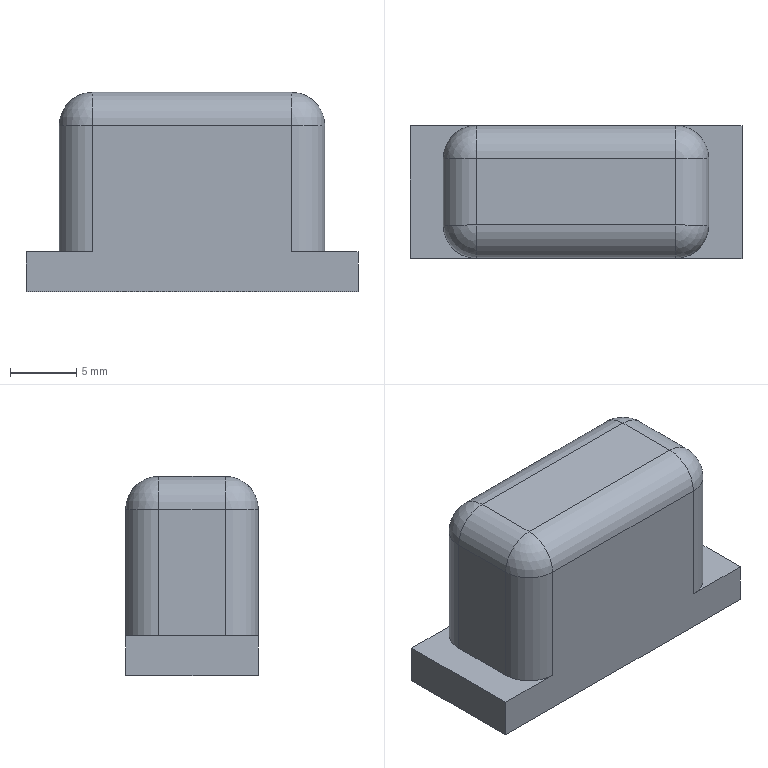NC program | NX | posted with a generic post | part box 25 x 10 x 15 mm
Lines 1366 to 3091 of 3091, first 1419 of 1722 lines:
(ZLEVEL_PROFILE_COPY_1 , TOOL : D4R0.5)
N2712 T05 M6
N2714 G54
N2716 G17 G0 G90 X1.318 Y-4.221 S7500 M3
N2718 G43 Z30. H5
N2720 Z1.
N2722 G94 G1 X-7.5 Z0.538 F1000.
N2724 X-7.686 Z0.528
N2726 X-8.139 Y-4.108 Z0.504
N2728 X-8.546 Y-3.879 Z0.479
N2730 X-8.877 Y-3.548 Z0.455
N2732 X-9.108 Y-3.142 Z0.43
N2734 X-9.221 Y-2.688 Z0.406
N2736 Y-2.502 Z0.396
N2738 Y2.502 Z0.134
N2740 Y2.688 Z0.124
N2742 X-9.108 Y3.141 Z0.099
N2744 X-8.878 Y3.547 Z0.075
N2746 X-8.548 Y3.877 Z0.051
N2748 X-8.142 Y4.107 Z0.026
N2750 X-7.689 Y4.221 Z0.002
N2752 X-7.503 Z-0.008
N2754 X7.503 F3000.
N2756 G2 X9.221 Y2.5 R1.721
N2758 G1 Y-2.5
N2760 G2 X7.5 Y-4.221 R1.721
N2762 G1 X-7.5
N2764 G2 X-9.221 Y-2.502 R1.721
N2766 G1 Y2.502
N2768 G2 X-7.503 Y4.221 R1.721
N2770 G1 X-7.401 Y4.244 Z-0.01
N2772 X-7.298 Y4.265 Z-0.012
N2774 X-7.195 Y4.285 Z-0.014
N2776 X-7.093 Y4.303 Z-0.015
N2778 X-6.99 Y4.32 Z-0.017
N2780 X-6.887 Y4.336 Z-0.019
N2782 X7.492
N2784 G2 X9.336 Y2.5 R1.836
N2786 G1 Y-2.5
N2788 G2 X7.5 Y-4.336 R1.836
N2790 G1 X-7.5
N2792 G2 X-9.336 Y-2.502 R1.836
N2794 G1 Y2.502
N2796 G2 X-7.504 Y4.336 R1.836
N2798 G1 X-7.367 Y4.357 Z-0.021
N2800 X-7.231 Y4.376 Z-0.024
N2802 X-7.094 Y4.394 Z-0.026
N2804 X-6.958 Y4.412 Z-0.028
N2806 X-6.821 Y4.429 Z-0.031
N2808 X-6.685 Y4.445 Z-0.033
N2810 X7.497
N2812 G2 X9.445 Y2.5 R1.945
N2814 G1 Y-2.5
N2816 G2 X7.5 Y-4.445 R1.945
N2818 G1 X-7.5
N2820 G2 X-9.445 Y-2.502 R1.945
N2822 G1 Y2.502
N2824 G2 X-7.504 Y4.445 R1.945
N2826 G1 X-7.379 Y4.459 Z-0.035
N2828 X-7.254 Y4.473 Z-0.038
N2830 X-7.129 Y4.487 Z-0.04
N2832 X-7.004 Y4.5 Z-0.042
N2834 X-6.88 Y4.512 Z-0.044
N2836 X-6.755 Y4.525 Z-0.046
N2838 X-6.63 Y4.537 Z-0.048
N2840 X-6.505 Y4.549 Z-0.051
N2842 X7.493
N2844 G2 X9.549 Y2.5 R2.049
N2846 G1 Y-2.5
N2848 G2 X7.5 Y-4.549 R2.049
N2850 G1 X-7.5
N2852 G2 X-9.549 Y-2.502 R2.049
N2854 G1 Y2.502
N2856 G2 X-7.504 Y4.549 R2.049
N2858 G1 X-7.385 Y4.56 Z-0.053
N2860 X-7.266 Y4.571 Z-0.055
N2862 X-7.146 Y4.581 Z-0.057
N2864 X-7.027 Y4.592 Z-0.059
N2866 X-6.908 Y4.602 Z-0.061
N2868 X-6.788 Y4.612 Z-0.063
N2870 X-6.669 Y4.622 Z-0.065
N2872 X-6.55 Y4.632 Z-0.067
N2874 X-6.431 Y4.641 Z-0.069
N2876 X-6.311 Y4.651 Z-0.071
N2878 X7.497
N2880 G2 X9.651 Y2.5 R2.151
N2882 G1 Y-2.5
N2884 G2 X7.5 Y-4.651 R2.151
N2886 G1 X-7.5
N2888 G2 X-9.651 Y-2.502 R2.151
N2890 G1 Y2.502
N2892 G2 X-7.504 Y4.651 R2.151
N2894 G1 X-7.366 Y4.662 Z-0.074
N2896 X-7.229 Y4.672 Z-0.076
N2898 X-7.091 Y4.683 Z-0.079
N2900 X-6.953 Y4.693 Z-0.081
N2902 X-6.815 Y4.703 Z-0.083
N2904 X-6.677 Y4.713 Z-0.086
N2906 X-6.539 Y4.722 Z-0.088
N2908 X-6.401 Y4.732 Z-0.091
N2910 X-6.263 Y4.742 Z-0.093
N2912 X-6.125 Y4.751 Z-0.096
N2914 X7.507
N2916 G2 X9.751 Y2.5 R2.251
N2918 G1 Y-2.5
N2920 G2 X7.5 Y-4.751 R2.251
N2922 G1 X-7.5
N2924 G2 X-9.751 Y-2.502 R2.251
N2926 G1 Y2.502
N2928 G2 X-7.507 Y4.751 R2.251
N2930 G1 X-7.504
N2932 X-7.374 Y4.76 Z-0.098
N2934 X-7.244 Y4.768 Z-0.1
N2936 X-7.114 Y4.777 Z-0.102
N2938 X-6.984 Y4.785 Z-0.105
N2940 X-6.854 Y4.794 Z-0.107
N2942 X-6.724 Y4.802 Z-0.109
N2944 X-6.594 Y4.81 Z-0.111
N2946 X-6.463 Y4.818 Z-0.114
N2948 X-6.333 Y4.826 Z-0.116
N2950 X-6.203 Y4.834 Z-0.118
N2952 X-6.073 Y4.842 Z-0.121
N2954 X-5.943 Y4.849 Z-0.123
N2956 X7.493
N2958 G2 X9.849 Y2.5 R2.349
N2960 G1 Y-2.5
N2962 G2 X7.5 Y-4.849 R2.349
N2964 G1 X-7.5
N2966 G2 X-9.849 Y-2.502 R2.349
N2968 G1 Y2.502
N2970 G2 X-7.505 Y4.849 R2.349
N2972 G1 X-7.38 Y4.857 Z-0.125
N2974 X-7.255 Y4.864 Z-0.127
N2976 X-7.131 Y4.871 Z-0.129
N2978 X-7.006 Y4.878 Z-0.131
N2980 X-6.881 Y4.885 Z-0.134
N2982 X-6.757 Y4.892 Z-0.136
N2984 X-6.632 Y4.899 Z-0.138
N2986 X-6.507 Y4.906 Z-0.14
N2988 X-6.383 Y4.913 Z-0.142
N2990 X-6.258 Y4.92 Z-0.145
N2992 X-6.134 Y4.927 Z-0.147
N2994 X-6.009 Y4.933 Z-0.149
N2996 X-5.884 Y4.94 Z-0.151
N2998 X-5.76 Y4.947 Z-0.153
N3000 X7.497
N3002 G2 X9.947 Y2.5 R2.447
N3004 G1 Y-2.5
N3006 G2 X7.5 Y-4.947 R2.447
N3008 G1 X-7.5
N3010 G2 X-9.947 Y-2.502 R2.447
N3012 G1 Y2.502
N3014 G2 X-7.505 Y4.947 R2.447
N3016 G1 X-7.367 Y4.954 Z-0.156
N3018 X-7.23 Y4.961 Z-0.158
N3020 X-7.092 Y4.968 Z-0.16
N3022 X-6.955 Y4.975 Z-0.163
N3024 X-6.817 Y4.982 Z-0.165
N3026 X-6.68 Y4.989 Z-0.168
N3028 X-6.542 Y4.996 Z-0.17
N3030 X-6.405 Y5.002 Z-0.172
N3032 X-6.267 Y5.009 Z-0.175
N3034 X-6.129 Y5.016 Z-0.177
N3036 X-5.992 Y5.023 Z-0.18
N3038 X-5.854 Y5.029 Z-0.182
N3040 X-5.717 Y5.036 Z-0.184
N3042 X-5.579 Y5.042 Z-0.187
N3044 X7.508
N3046 G2 X10.042 Y2.5 R2.542
N3048 G1 Y-2.5
N3050 G2 X7.5 Y-5.042 R2.542
N3052 G1 X-7.5
N3054 G2 X-10.042 Y-2.502 R2.542
N3056 G1 Y2.502
N3058 G2 X-7.508 Y5.042 R2.542
N3060 G1 X-7.505
N3062 X-7.373 Y5.048 Z-0.189
N3064 X-7.242 Y5.054 Z-0.191
N3066 X-7.11 Y5.061 Z-0.194
N3068 X-6.979 Y5.067 Z-0.196
N3070 X-6.847 Y5.073 Z-0.198
N3072 X-6.715 Y5.079 Z-0.201
N3074 X-6.584 Y5.085 Z-0.203
N3076 X-6.452 Y5.09 Z-0.205
N3078 X-6.321 Y5.096 Z-0.208
N3080 X-6.189 Y5.102 Z-0.21
N3082 X-6.058 Y5.108 Z-0.212
N3084 X-5.926 Y5.114 Z-0.214
N3086 X-5.795 Y5.119 Z-0.217
N3088 X-5.663 Y5.125 Z-0.219
N3090 X-5.531 Y5.131 Z-0.221
N3092 X-5.4 Y5.136 Z-0.224
N3094 X7.494
N3096 G2 X10.136 Y2.5 R2.636
N3098 G1 Y-2.5
N3100 G2 X7.5 Y-5.136 R2.636
N3102 G1 X-7.5
N3104 G2 X-10.136 Y-2.502 R2.636
N3106 G1 Y2.502
N3108 G2 X-7.505 Y5.136 R2.636
N3110 G1 X-7.378 Y5.142 Z-0.226
N3112 X-7.252 Y5.147 Z-0.228
N3114 X-7.125 Y5.153 Z-0.23
N3116 X-6.998 Y5.158 Z-0.232
N3118 X-6.871 Y5.163 Z-0.235
N3120 X-6.745 Y5.168 Z-0.237
N3122 X-6.618 Y5.174 Z-0.239
N3124 X-6.491 Y5.179 Z-0.241
N3126 X-6.364 Y5.184 Z-0.243
N3128 X-6.238 Y5.189 Z-0.246
N3130 X-6.111 Y5.194 Z-0.248
N3132 X-5.984 Y5.199 Z-0.25
N3134 X-5.858 Y5.204 Z-0.252
N3136 X-5.731 Y5.209 Z-0.255
N3138 X-5.604 Y5.214 Z-0.257
N3140 X-5.477 Y5.219 Z-0.259
N3142 X-5.351 Y5.224 Z-0.261
N3144 X-5.224 Y5.229 Z-0.263
N3146 X7.497
N3148 G2 X10.229 Y2.5 R2.729
N3150 G1 Y-2.5
N3152 G2 X7.5 Y-5.229 R2.729
N3154 G1 X-7.5
N3156 G2 X-10.229 Y-2.502 R2.729
N3158 G1 Y2.502
N3160 G2 X-7.505 Y5.229 R2.729
N3162 G1 X-7.369 Y5.235 Z-0.266
N3164 X-7.232 Y5.24 Z-0.268
N3166 X-7.096 Y5.245 Z-0.271
N3168 X-6.96 Y5.25 Z-0.273
N3170 X-6.823 Y5.255 Z-0.275
N3172 X-6.687 Y5.261 Z-0.278
N3174 X-6.551 Y5.266 Z-0.28
N3176 X-6.414 Y5.271 Z-0.282
N3178 X-6.278 Y5.276 Z-0.285
N3180 X-6.141 Y5.281 Z-0.287
N3182 X-6.005 Y5.286 Z-0.29
N3184 X-5.869 Y5.291 Z-0.292
N3186 X-5.732 Y5.296 Z-0.294
N3188 X-5.596 Y5.301 Z-0.297
N3190 X-5.46 Y5.306 Z-0.299
N3192 X-5.323 Y5.311 Z-0.301
N3194 X-5.187 Y5.316 Z-0.304
N3196 X-5.051 Y5.32 Z-0.306
N3198 X7.491
N3200 G2 X10.32 Y2.5 R2.82
N3202 G1 Y-2.5
N3204 G2 X7.5 Y-5.32 R2.82
N3206 G1 X-7.5
N3208 G2 X-10.32 Y-2.502 R2.82
N3210 G1 Y2.502
N3212 G2 X-7.505 Y5.32 R2.82
N3214 G1 X-7.374 Y5.325 Z-0.309
N3216 X-7.243 Y5.33 Z-0.311
N3218 X-7.111 Y5.334 Z-0.313
N3220 X-6.98 Y5.339 Z-0.315
N3222 X-6.849 Y5.344 Z-0.318
N3224 X-6.717 Y5.348 Z-0.32
N3226 X-6.586 Y5.353 Z-0.322
N3228 X-6.455 Y5.357 Z-0.325
N3230 X-6.324 Y5.362 Z-0.327
N3232 X-6.192 Y5.366 Z-0.329
N3234 X-6.061 Y5.371 Z-0.331
N3236 X-5.93 Y5.375 Z-0.334
N3238 X-5.798 Y5.38 Z-0.336
N3240 X-5.667 Y5.384 Z-0.338
N3242 X-5.536 Y5.388 Z-0.341
N3244 X-5.404 Y5.393 Z-0.343
N3246 X-5.273 Y5.397 Z-0.345
N3248 X-5.142 Y5.401 Z-0.347
N3250 X-5.011 Y5.406 Z-0.35
N3252 X-4.879 Y5.41 Z-0.352
N3254 X7.494
N3256 G2 X10.41 Y2.5 R2.91
N3258 G1 Y-2.5
N3260 G2 X7.5 Y-5.41 R2.91
N3262 G1 X-7.5
N3264 G2 X-10.41 Y-2.502 R2.91
N3266 G1 Y2.502
N3268 G2 X-7.505 Y5.41 R2.91
N3270 G1 X-7.366 Y5.415 Z-0.355
N3272 X-7.226 Y5.419 Z-0.357
N3274 X-7.086 Y5.424 Z-0.359
N3276 X-6.947 Y5.428 Z-0.362
N3278 X-6.807 Y5.433 Z-0.364
N3280 X-6.667 Y5.437 Z-0.367
N3282 X-6.528 Y5.442 Z-0.369
N3284 X-6.388 Y5.446 Z-0.372
N3286 X-6.248 Y5.451 Z-0.374
N3288 X-6.108 Y5.455 Z-0.376
N3290 X-5.969 Y5.459 Z-0.379
N3292 X-5.829 Y5.464 Z-0.381
N3294 X-5.689 Y5.468 Z-0.384
N3296 X-5.55 Y5.472 Z-0.386
N3298 X-5.41 Y5.477 Z-0.389
N3300 X-5.27 Y5.481 Z-0.391
N3302 X-5.131 Y5.485 Z-0.394
N3304 X-4.991 Y5.49 Z-0.396
N3306 X-4.851 Y5.494 Z-0.398
N3308 X-4.711 Y5.498 Z-0.401
N3310 X7.497
N3312 G2 X10.498 Y2.5 R2.998
N3314 G1 Y-2.5
N3316 G2 X7.5 Y-5.498 R2.998
N3318 G1 X-7.5
N3320 G2 X-10.498 Y-2.502 R2.998
N3322 G1 Y2.502
N3324 G2 X-7.506 Y5.498 R2.998
N3326 G1 X-7.371 Y5.502 Z-0.403
N3328 X-7.237 Y5.506 Z-0.406
N3330 X-7.102 Y5.51 Z-0.408
N3332 X-6.968 Y5.514 Z-0.41
N3334 X-6.833 Y5.518 Z-0.413
N3336 X-6.698 Y5.522 Z-0.415
N3338 X-6.564 Y5.526 Z-0.417
N3340 X-6.429 Y5.53 Z-0.42
N3342 X-6.295 Y5.534 Z-0.422
N3344 X-6.16 Y5.538 Z-0.424
N3346 X-6.026 Y5.542 Z-0.427
N3348 X-5.891 Y5.546 Z-0.429
N3350 X-5.757 Y5.55 Z-0.431
N3352 X-5.622 Y5.554 Z-0.434
N3354 X-5.488 Y5.558 Z-0.436
N3356 X-5.353 Y5.562 Z-0.438
N3358 X-5.219 Y5.565 Z-0.441
N3360 X-5.084 Y5.569 Z-0.443
N3362 X-4.95 Y5.573 Z-0.445
N3364 X-4.815 Y5.577 Z-0.448
N3366 X-4.681 Y5.581 Z-0.45
N3368 X-4.546 Y5.584 Z-0.453
N3370 X7.507
N3372 G2 X10.584 Y2.5 R3.084
N3374 G1 Y-2.5
N3376 G2 X7.5 Y-5.584 R3.084
N3378 G1 X-7.5
N3380 G2 X-10.584 Y-2.502 R3.084
N3382 G1 Y2.502
N3384 G2 X-7.507 Y5.584 R3.084
N3386 G1 X-7.506
N3388 X-7.376 Y5.588 Z-0.455
N3390 X-7.246 Y5.592 Z-0.457
N3392 X-7.116 Y5.595 Z-0.459
N3394 X-6.985 Y5.599 Z-0.462
N3396 X-6.855 Y5.602 Z-0.464
N3398 X-6.725 Y5.606 Z-0.466
N3400 X-6.595 Y5.61 Z-0.468
N3402 X-6.465 Y5.613 Z-0.471
N3404 X-6.335 Y5.617 Z-0.473
N3406 X-6.205 Y5.62 Z-0.475
N3408 X-6.075 Y5.624 Z-0.477
N3410 X-5.945 Y5.627 Z-0.48
N3412 X-5.815 Y5.631 Z-0.482
N3414 X-5.685 Y5.634 Z-0.484
N3416 X-5.555 Y5.638 Z-0.487
N3418 X-5.425 Y5.641 Z-0.489
N3420 X-5.295 Y5.645 Z-0.491
N3422 X-5.165 Y5.648 Z-0.493
N3424 X-5.035 Y5.652 Z-0.496
N3426 X-4.905 Y5.655 Z-0.498
N3428 X-4.775 Y5.659 Z-0.5
N3430 X-4.645 Y5.662 Z-0.502
N3432 X-4.515 Y5.665 Z-0.505
N3434 X-4.385 Y5.669 Z-0.507
N3436 X7.492
N3438 G2 X10.669 Y2.5 R3.169
N3440 G1 Y-2.5
N3442 G2 X7.5 Y-5.669 R3.169
N3444 G1 X-7.5
N3446 G2 X-10.669 Y-2.502 R3.169
N3448 G1 Y2.502
N3450 G2 X-7.506 Y5.669 R3.169
N3452 G1 X-7.369 Y5.672 Z-0.509
N3454 X-7.232 Y5.676 Z-0.512
N3456 X-7.096 Y5.679 Z-0.514
N3458 X-6.959 Y5.683 Z-0.517
N3460 X-6.822 Y5.686 Z-0.519
N3462 X-6.686 Y5.69 Z-0.521
N3464 X-6.549 Y5.693 Z-0.524
N3466 X-6.412 Y5.697 Z-0.526
N3468 X-6.276 Y5.7 Z-0.528
N3470 X-6.139 Y5.704 Z-0.531
N3472 X-6.003 Y5.707 Z-0.533
N3474 X-5.866 Y5.711 Z-0.536
N3476 X-5.729 Y5.714 Z-0.538
N3478 X-5.593 Y5.718 Z-0.54
N3480 X-5.456 Y5.721 Z-0.543
N3482 X-5.319 Y5.724 Z-0.545
N3484 X-5.183 Y5.728 Z-0.548
N3486 X-5.046 Y5.731 Z-0.55
N3488 X-4.909 Y5.735 Z-0.552
N3490 X-4.773 Y5.738 Z-0.555
N3492 X-4.636 Y5.741 Z-0.557
N3494 X-4.499 Y5.745 Z-0.559
N3496 X-4.363 Y5.748 Z-0.562
N3498 X-4.226 Y5.751 Z-0.564
N3500 X7.495
N3502 G2 X10.751 Y2.5 R3.251
N3504 G1 Y-2.5
N3506 G2 X7.5 Y-5.751 R3.251
N3508 G1 X-7.5
N3510 G2 X-10.751 Y-2.502 R3.251
N3512 G1 Y2.502
N3514 G2 X-7.506 Y5.751 R3.251
N3516 G1 X-7.374 Y5.754 Z-0.567
N3518 X-7.242 Y5.758 Z-0.569
N3520 X-7.11 Y5.761 Z-0.571
N3522 X-6.978 Y5.764 Z-0.573
N3524 X-6.845 Y5.767 Z-0.576
N3526 X-6.713 Y5.77 Z-0.578
N3528 X-6.581 Y5.774 Z-0.58
N3530 X-6.449 Y5.777 Z-0.583
N3532 X-6.317 Y5.78 Z-0.585
N3534 X-6.185 Y5.783 Z-0.587
N3536 X-6.053 Y5.786 Z-0.59
N3538 X-5.921 Y5.789 Z-0.592
N3540 X-5.789 Y5.792 Z-0.594
N3542 X-5.657 Y5.795 Z-0.597
N3544 X-5.525 Y5.798 Z-0.599
N3546 X-5.393 Y5.801 Z-0.601
N3548 X-5.26 Y5.805 Z-0.603
N3550 X-5.128 Y5.808 Z-0.606
N3552 X-4.996 Y5.811 Z-0.608
N3554 X-4.864 Y5.814 Z-0.61
N3556 X-4.732 Y5.817 Z-0.613
N3558 X-4.6 Y5.82 Z-0.615
N3560 X-4.468 Y5.823 Z-0.617
N3562 X-4.336 Y5.826 Z-0.62
N3564 X-4.204 Y5.829 Z-0.622
N3566 X-4.072 Y5.832 Z-0.624
N3568 X7.497
N3570 G2 X10.832 Y2.5 R3.332
N3572 G1 Y-2.5
N3574 G2 X7.5 Y-5.832 R3.332
N3576 G1 X-7.5
N3578 G2 X-10.832 Y-2.502 R3.332
N3580 G1 Y2.502
N3582 G2 X-7.506 Y5.832 R3.332
N3584 G1 X-7.368 Y5.835 Z-0.627
N3586 X-7.23 Y5.838 Z-0.629
N3588 X-7.092 Y5.841 Z-0.631
N3590 X-6.955 Y5.844 Z-0.634
N3592 X-6.817 Y5.847 Z-0.636
N3594 X-6.679 Y5.85 Z-0.639
N3596 X-6.541 Y5.853 Z-0.641
N3598 X-6.403 Y5.856 Z-0.643
N3600 X-6.265 Y5.86 Z-0.646
N3602 X-6.127 Y5.863 Z-0.648
N3604 X-5.989 Y5.866 Z-0.651
N3606 X-5.851 Y5.869 Z-0.653
N3608 X-5.714 Y5.872 Z-0.655
N3610 X-5.576 Y5.875 Z-0.658
N3612 X-5.438 Y5.878 Z-0.66
N3614 X-5.3 Y5.881 Z-0.663
N3616 X-5.162 Y5.884 Z-0.665
N3618 X-5.024 Y5.887 Z-0.667
N3620 X-4.886 Y5.89 Z-0.67
N3622 X-4.748 Y5.893 Z-0.672
N3624 X-4.611 Y5.896 Z-0.675
N3626 X-4.473 Y5.898 Z-0.677
N3628 X-4.335 Y5.901 Z-0.68
N3630 X-4.197 Y5.904 Z-0.682
N3632 X-4.059 Y5.907 Z-0.684
N3634 X-3.921 Y5.91 Z-0.687
N3636 X7.509
N3638 G2 X10.91 Y2.5 R3.41
N3640 G1 Y-2.5
N3642 G2 X7.5 Y-5.91 R3.41
N3644 G1 X-7.5
N3646 G2 X-10.91 Y-2.502 R3.41
N3648 G1 Y2.502
N3650 G2 X-7.509 Y5.91 R3.41
N3652 G1 X-7.506
N3654 X-7.373 Y5.913 Z-0.689
N3656 X-7.239 Y5.916 Z-0.691
N3658 X-7.106 Y5.919 Z-0.694
N3660 X-6.973 Y5.921 Z-0.696
N3662 X-6.84 Y5.924 Z-0.698
N3664 X-6.706 Y5.927 Z-0.701
N3666 X-6.573 Y5.93 Z-0.703
N3668 X-6.44 Y5.933 Z-0.705
N3670 X-6.306 Y5.935 Z-0.708
N3672 X-6.173 Y5.938 Z-0.71
N3674 X-6.04 Y5.941 Z-0.712
N3676 X-5.906 Y5.944 Z-0.715
N3678 X-5.773 Y5.946 Z-0.717
N3680 X-5.64 Y5.949 Z-0.719
N3682 X-5.507 Y5.952 Z-0.722
N3684 X-5.373 Y5.954 Z-0.724
N3686 X-5.24 Y5.957 Z-0.726
N3688 X-5.107 Y5.96 Z-0.729
N3690 X-4.973 Y5.963 Z-0.731
N3692 X-4.84 Y5.965 Z-0.733
N3694 X-4.707 Y5.968 Z-0.736
N3696 X-4.573 Y5.971 Z-0.738
N3698 X-4.44 Y5.973 Z-0.74
N3700 X-4.307 Y5.976 Z-0.743
N3702 X-4.174 Y5.979 Z-0.745
N3704 X-4.04 Y5.981 Z-0.747
N3706 X-3.907 Y5.984 Z-0.75
N3708 X-3.774 Y5.986 Z-0.752
N3710 X7.493
N3712 G2 X10.986 Y2.5 R3.486
N3714 G1 Y-2.5
N3716 G2 X7.5 Y-5.986 R3.486
N3718 G1 X-7.5
N3720 G2 X-10.986 Y-2.502 R3.486
N3722 G1 Y2.502
N3724 G2 X-7.506 Y5.986 R3.486
N3726 G1 X-7.368 Y5.989 Z-0.754
N3728 X-7.229 Y5.992 Z-0.757
N3730 X-7.091 Y5.995 Z-0.759
N3732 X-6.953 Y5.997 Z-0.762
N3734 X-6.814 Y6. Z-0.764
N3736 X-6.676 Y6.003 Z-0.766
N3738 X-6.538 Y6.005 Z-0.769
N3740 X-6.399 Y6.008 Z-0.771
N3742 X-6.261 Y6.011 Z-0.774
N3744 X-6.122 Y6.013 Z-0.776
N3746 X-5.984 Y6.016 Z-0.778
N3748 X-5.846 Y6.019 Z-0.781
N3750 X-5.707 Y6.021 Z-0.783
N3752 X-5.569 Y6.024 Z-0.786
N3754 X-5.43 Y6.027 Z-0.788
N3756 X-5.292 Y6.029 Z-0.791
N3758 X-5.154 Y6.032 Z-0.793
N3760 X-5.015 Y6.035 Z-0.795
N3762 X-4.877 Y6.037 Z-0.798
N3764 X-4.739 Y6.04 Z-0.8
N3766 X-4.6 Y6.042 Z-0.803
N3768 X-4.462 Y6.045 Z-0.805
N3770 X-4.323 Y6.048 Z-0.807
N3772 X-4.185 Y6.05 Z-0.81
N3774 X-4.047 Y6.053 Z-0.812
N3776 X-3.908 Y6.055 Z-0.815
N3778 X-3.77 Y6.058 Z-0.817
N3780 X-3.631 Y6.06 Z-0.82
N3782 X7.495
N3784 G2 X11.06 Y2.5 R3.56
N3786 G1 Y-2.5
N3788 G2 X7.5 Y-6.06 R3.56
N3790 G1 X-7.5
N3792 G2 X-11.06 Y-2.502 R3.56
N3794 G1 Y2.502
N3796 G2 X-7.506 Y6.06 R3.56
N3798 G1 X-7.373 Y6.063 Z-0.822
N3800 X-7.239 Y6.065 Z-0.824
N3802 X-7.105 Y6.068 Z-0.827
N3804 X-6.971 Y6.07 Z-0.829
N3806 X-6.837 Y6.073 Z-0.831
N3808 X-6.704 Y6.075 Z-0.834
N3810 X-6.57 Y6.078 Z-0.836
N3812 X-6.436 Y6.08 Z-0.838
N3814 X-6.302 Y6.082 Z-0.841
N3816 X-6.169 Y6.085 Z-0.843
N3818 X-6.035 Y6.087 Z-0.845
N3820 X-5.901 Y6.09 Z-0.848
N3822 X-5.767 Y6.092 Z-0.85
N3824 X-5.633 Y6.095 Z-0.852
N3826 X-5.5 Y6.097 Z-0.855
N3828 X-5.366 Y6.099 Z-0.857
N3830 X-5.232 Y6.102 Z-0.859
N3832 X-5.098 Y6.104 Z-0.862
N3834 X-4.965 Y6.106 Z-0.864
N3836 X-4.831 Y6.109 Z-0.866
N3838 X-4.697 Y6.111 Z-0.869
N3840 X-4.563 Y6.114 Z-0.871
N3842 X-4.429 Y6.116 Z-0.873
N3844 X-4.296 Y6.118 Z-0.876
N3846 X-4.162 Y6.121 Z-0.878
N3848 X-4.028 Y6.123 Z-0.88
N3850 X-3.894 Y6.125 Z-0.883
N3852 X-3.761 Y6.128 Z-0.885
N3854 X-3.627 Y6.13 Z-0.887
N3856 X-3.493 Y6.132 Z-0.89
N3858 X7.497
N3860 G2 X11.132 Y2.5 R3.632
N3862 G1 Y-2.5
N3864 G2 X7.5 Y-6.132 R3.632
N3866 G1 X-7.5
N3868 G2 X-11.132 Y-2.502 R3.632
N3870 G1 Y2.502
N3872 G2 X-7.506 Y6.132 R3.632
N3874 G1 X-7.368 Y6.135 Z-0.892
N3876 X-7.23 Y6.137 Z-0.894
N3878 X-7.092 Y6.139 Z-0.897
N3880 X-6.953 Y6.142 Z-0.899
N3882 X-6.815 Y6.144 Z-0.902
N3884 X-6.677 Y6.146 Z-0.904
N3886 X-6.539 Y6.149 Z-0.906
N3888 X-6.4 Y6.151 Z-0.909
N3890 X-6.262 Y6.153 Z-0.911
N3892 X-6.124 Y6.156 Z-0.914
N3894 X-5.986 Y6.158 Z-0.916
N3896 X-5.847 Y6.16 Z-0.919
N3898 X-5.709 Y6.163 Z-0.921
N3900 X-5.571 Y6.165 Z-0.923
N3902 X-5.433 Y6.167 Z-0.926
N3904 X-5.294 Y6.17 Z-0.928
N3906 X-5.156 Y6.172 Z-0.931
N3908 X-5.018 Y6.174 Z-0.933
N3910 X-4.88 Y6.177 Z-0.935
N3912 X-4.741 Y6.179 Z-0.938
N3914 X-4.603 Y6.181 Z-0.94
N3916 X-4.465 Y6.183 Z-0.943
N3918 X-4.327 Y6.186 Z-0.945
N3920 X-4.189 Y6.188 Z-0.948
N3922 X-4.05 Y6.19 Z-0.95
N3924 X-3.912 Y6.192 Z-0.952
N3926 X-3.774 Y6.195 Z-0.955
N3928 X-3.636 Y6.197 Z-0.957
N3930 X-3.497 Y6.199 Z-0.96
N3932 X-3.359 Y6.201 Z-0.962
N3934 X7.492
N3936 G2 X11.201 Y2.5 R3.701
N3938 G1 Y-2.5
N3940 G2 X7.5 Y-6.201 R3.701
N3942 G1 X-7.5
N3944 G2 X-11.201 Y-2.502 R3.701
N3946 G1 Y2.502
N3948 G2 X-7.507 Y6.201 R3.701
N3950 G1 X-7.373 Y6.204 Z-0.964
N3952 X-7.239 Y6.206 Z-0.967
N3954 X-7.106 Y6.208 Z-0.969
N3956 X-6.972 Y6.21 Z-0.971
N3958 X-6.838 Y6.212 Z-0.974
N3960 X-6.705 Y6.214 Z-0.976
N3962 X-6.571 Y6.216 Z-0.978
N3964 X-6.437 Y6.219 Z-0.981
N3966 X-6.304 Y6.221 Z-0.983
N3968 X-6.17 Y6.223 Z-0.985
N3970 X-6.037 Y6.225 Z-0.988
N3972 X-5.903 Y6.227 Z-0.99
N3974 X-5.769 Y6.229 Z-0.992
N3976 X-5.636 Y6.231 Z-0.995
N3978 X-5.502 Y6.233 Z-0.997
N3980 X-5.368 Y6.235 Z-0.999
N3982 X-5.235 Y6.238 Z-1.002
N3984 X-5.101 Y6.24 Z-1.004
N3986 X-4.967 Y6.242 Z-1.006
N3988 X-4.834 Y6.244 Z-1.009
N3990 X-4.7 Y6.246 Z-1.011
N3992 X-4.566 Y6.248 Z-1.013
N3994 X-4.433 Y6.25 Z-1.016
N3996 X-4.299 Y6.252 Z-1.018
N3998 X-4.166 Y6.254 Z-1.02
N4000 X-4.032 Y6.256 Z-1.023
N4002 X-3.898 Y6.258 Z-1.025
N4004 X-3.765 Y6.26 Z-1.027
N4006 X-3.631 Y6.262 Z-1.03
N4008 X-3.497 Y6.264 Z-1.032
N4010 X-3.364 Y6.266 Z-1.034
N4012 X-3.23 Y6.268 Z-1.037
N4014 X7.494
N4016 G2 X11.268 Y2.5 R3.768
N4018 G1 Y-2.5
N4020 G2 X7.5 Y-6.268 R3.768
N4022 G1 X-7.5
N4024 G2 X-11.268 Y-2.502 R3.768
N4026 G1 Y2.502
N4028 G2 X-7.507 Y6.268 R3.768
N4030 G1 X-7.369 Y6.27 Z-1.039
N4032 X-7.232 Y6.272 Z-1.041
N4034 X-7.094 Y6.275 Z-1.044
N4036 X-6.956 Y6.277 Z-1.046
N4038 X-6.819 Y6.279 Z-1.049
N4040 X-6.681 Y6.281 Z-1.051
N4042 X-6.544 Y6.283 Z-1.053
N4044 X-6.406 Y6.285 Z-1.056
N4046 X-6.269 Y6.287 Z-1.058
N4048 X-6.131 Y6.289 Z-1.061
N4050 X-5.994 Y6.291 Z-1.063
N4052 X-5.856 Y6.293 Z-1.065
N4054 X-5.719 Y6.295 Z-1.068
N4056 X-5.581 Y6.297 Z-1.07
N4058 X-5.443 Y6.299 Z-1.073
N4060 X-5.306 Y6.301 Z-1.075
N4062 X-5.168 Y6.303 Z-1.077
N4064 X-5.031 Y6.305 Z-1.08
N4066 X-4.893 Y6.307 Z-1.082
N4068 X-4.756 Y6.309 Z-1.085
N4070 X-4.618 Y6.311 Z-1.087
N4072 X-4.481 Y6.313 Z-1.089
N4074 X-4.343 Y6.315 Z-1.092
N4076 X-4.205 Y6.317 Z-1.094
N4078 X-4.068 Y6.319 Z-1.097
N4080 X-3.93 Y6.321 Z-1.099
N4082 X-3.793 Y6.323 Z-1.101
N4084 X-3.655 Y6.325 Z-1.104
N4086 X-3.518 Y6.327 Z-1.106
N4088 X-3.38 Y6.329 Z-1.109
N4090 X-3.243 Y6.331 Z-1.111
N4092 X-3.105 Y6.333 Z-1.113
N4094 X7.496
N4096 G2 X11.333 Y2.5 R3.833
N4098 G1 Y-2.5
N4100 G2 X7.5 Y-6.333 R3.833
N4102 G1 X-7.5
N4104 G2 X-11.333 Y-2.502 R3.833
N4106 G1 Y2.502
N4108 G2 X-7.507 Y6.333 R3.833
N4110 G1 X-7.366 Y6.335 Z-1.116
N4112 X-7.224 Y6.337 Z-1.118
N4114 X-7.083 Y6.339 Z-1.121
N4116 X-6.942 Y6.341 Z-1.123
N4118 X-6.8 Y6.343 Z-1.126
N4120 X-6.659 Y6.344 Z-1.128
N4122 X-6.518 Y6.346 Z-1.131
N4124 X-6.377 Y6.348 Z-1.133
N4126 X-6.235 Y6.35 Z-1.136
N4128 X-6.094 Y6.352 Z-1.138
N4130 X-5.953 Y6.354 Z-1.141
N4132 X-5.811 Y6.356 Z-1.143
N4134 X-5.67 Y6.358 Z-1.146
N4136 X-5.529 Y6.36 Z-1.148
N4138 X-5.387 Y6.362 Z-1.15
N4140 X-5.246 Y6.364 Z-1.153
N4142 X-5.105 Y6.366 Z-1.155
N4144 X-4.964 Y6.368 Z-1.158
N4146 X-4.822 Y6.37 Z-1.16
N4148 X-4.681 Y6.372 Z-1.163
N4150 X-4.54 Y6.374 Z-1.165
N4152 X-4.398 Y6.375 Z-1.168
N4154 X-4.257 Y6.377 Z-1.17
N4156 X-4.116 Y6.379 Z-1.173
N4158 X-3.975 Y6.381 Z-1.175
N4160 X-3.833 Y6.383 Z-1.178
N4162 X-3.692 Y6.385 Z-1.18
N4164 X-3.551 Y6.387 Z-1.183
N4166 X-3.409 Y6.389 Z-1.185
N4168 X-3.268 Y6.391 Z-1.187
N4170 X-3.127 Y6.392 Z-1.19
N4172 X-2.986 Y6.394 Z-1.192
N4174 X7.497
N4176 G2 X11.394 Y2.5 R3.894
N4178 G1 Y-2.5
N4180 G2 X7.5 Y-6.394 R3.894
N4182 G1 X-7.5
N4184 G2 X-11.394 Y-2.502 R3.894
N4186 G1 Y2.502
N4188 G2 X-7.507 Y6.394 R3.894
N4190 G1 X-7.371 Y6.396 Z-1.195
N4192 X-7.234 Y6.398 Z-1.197
N4194 X-7.098 Y6.4 Z-1.2
N4196 X-6.962 Y6.401 Z-1.202
N4198 X-6.825 Y6.403 Z-1.204
N4200 X-6.689 Y6.405 Z-1.207
N4202 X-6.552 Y6.407 Z-1.209
N4204 X-6.416 Y6.409 Z-1.211
N4206 X-6.28 Y6.41 Z-1.214
N4208 X-6.143 Y6.412 Z-1.216
N4210 X-6.007 Y6.414 Z-1.219
N4212 X-5.871 Y6.416 Z-1.221
N4214 X-5.734 Y6.417 Z-1.223
N4216 X-5.598 Y6.419 Z-1.226
N4218 X-5.462 Y6.421 Z-1.228
N4220 X-5.325 Y6.423 Z-1.23
N4222 X-5.189 Y6.424 Z-1.233
N4224 X-5.053 Y6.426 Z-1.235
N4226 X-4.916 Y6.428 Z-1.238
N4228 X-4.78 Y6.429 Z-1.24
N4230 X-4.644 Y6.431 Z-1.242
N4232 X-4.507 Y6.433 Z-1.245
N4234 X-4.371 Y6.435 Z-1.247
N4236 X-4.235 Y6.436 Z-1.249
N4238 X-4.098 Y6.438 Z-1.252
N4240 X-3.962 Y6.44 Z-1.254
N4242 X-3.825 Y6.441 Z-1.257
N4244 X-3.689 Y6.443 Z-1.259
N4246 X-3.553 Y6.445 Z-1.261
N4248 X-3.416 Y6.447 Z-1.264
N4250 X-3.28 Y6.448 Z-1.266
N4252 X-3.144 Y6.45 Z-1.269
N4254 X-3.007 Y6.452 Z-1.271
N4256 X-2.871 Y6.453 Z-1.273
N4258 X7.492
N4260 G2 X11.453 Y2.5 R3.953
N4262 G1 Y-2.5
N4264 G2 X7.5 Y-6.453 R3.953
N4266 G1 X-7.5
N4268 G2 X-11.453 Y-2.502 R3.953
N4270 G1 Y2.502
N4272 G2 X-7.507 Y6.453 R3.953
N4274 G1 X-7.367 Y6.455 Z-1.276
N4276 X-7.228 Y6.457 Z-1.278
N4278 X-7.088 Y6.458 Z-1.281
N4280 X-6.949 Y6.46 Z-1.283
N4282 X-6.809 Y6.462 Z-1.285
N4284 X-6.67 Y6.463 Z-1.288
N4286 X-6.53 Y6.465 Z-1.29
N4288 X-6.39 Y6.467 Z-1.293
N4290 X-6.251 Y6.469 Z-1.295
N4292 X-6.111 Y6.47 Z-1.298
N4294 X-5.972 Y6.472 Z-1.3
N4296 X-5.832 Y6.474 Z-1.303
N4298 X-5.693 Y6.475 Z-1.305
N4300 X-5.553 Y6.477 Z-1.307
N4302 X-5.413 Y6.479 Z-1.31
N4304 X-5.274 Y6.48 Z-1.312
N4306 X-5.134 Y6.482 Z-1.315
N4308 X-4.995 Y6.484 Z-1.317
N4310 X-4.855 Y6.485 Z-1.32
N4312 X-4.716 Y6.487 Z-1.322
N4314 X-4.576 Y6.488 Z-1.324
N4316 X-4.436 Y6.49 Z-1.327
N4318 X-4.297 Y6.492 Z-1.329
N4320 X-4.157 Y6.493 Z-1.332
N4322 X-4.018 Y6.495 Z-1.334
N4324 X-3.878 Y6.497 Z-1.337
N4326 X-3.739 Y6.498 Z-1.339
N4328 X-3.599 Y6.5 Z-1.342
N4330 X-3.459 Y6.501 Z-1.344
N4332 X-3.32 Y6.503 Z-1.346
N4334 X-3.18 Y6.505 Z-1.349
N4336 X-3.041 Y6.506 Z-1.351
N4338 X-2.901 Y6.508 Z-1.354
N4340 X-2.762 Y6.51 Z-1.356
N4342 X7.494
N4344 G2 X11.51 Y2.5 R4.01
N4346 G1 Y-2.5
N4348 G2 X7.5 Y-6.51 R4.01
N4350 G1 X-7.5
N4352 G2 X-11.51 Y-2.502 R4.01
N4354 G1 Y2.502
N4356 G2 X-7.507 Y6.51 R4.01
N4358 G1 X-7.372 Y6.511 Z-1.358
N4360 X-7.238 Y6.513 Z-1.361
N4362 X-7.103 Y6.514 Z-1.363
N4364 X-6.968 Y6.516 Z-1.366
N4366 X-6.834 Y6.517 Z-1.368
N4368 X-6.699 Y6.519 Z-1.37
N4370 X-6.564 Y6.52 Z-1.373
N4372 X-6.429 Y6.522 Z-1.375
N4374 X-6.295 Y6.523 Z-1.377
N4376 X-6.16 Y6.525 Z-1.38
N4378 X-6.025 Y6.526 Z-1.382
N4380 X-5.89 Y6.528 Z-1.384
N4382 X-5.756 Y6.529 Z-1.387
N4384 X-5.621 Y6.531 Z-1.389
N4386 X-5.486 Y6.532 Z-1.391
N4388 X-5.352 Y6.534 Z-1.394
N4390 X-5.217 Y6.535 Z-1.396
N4392 X-5.082 Y6.537 Z-1.398
N4394 X-4.947 Y6.538 Z-1.401
N4396 X-4.813 Y6.54 Z-1.403
N4398 X-4.678 Y6.541 Z-1.406
N4400 X-4.543 Y6.543 Z-1.408
N4402 X-4.409 Y6.544 Z-1.41
N4404 X-4.274 Y6.546 Z-1.413
N4406 X-4.139 Y6.547 Z-1.415
N4408 X-4.004 Y6.549 Z-1.417
N4410 X-3.87 Y6.55 Z-1.42
N4412 X-3.735 Y6.551 Z-1.422
N4414 X-3.6 Y6.553 Z-1.424
N4416 X-3.465 Y6.554 Z-1.427
N4418 X-3.331 Y6.556 Z-1.429
N4420 X-3.196 Y6.557 Z-1.431
N4422 X-3.061 Y6.559 Z-1.434
N4424 X-2.927 Y6.56 Z-1.436
N4426 X-2.792 Y6.562 Z-1.438
N4428 X-2.657 Y6.563 Z-1.441
N4430 X7.495
N4432 G2 X11.563 Y2.5 R4.063
N4434 G1 Y-2.5
N4436 G2 X7.5 Y-6.563 R4.063
N4438 G1 X-7.5
N4440 G2 X-11.563 Y-2.502 R4.063
N4442 G1 Y2.502
N4444 G2 X-7.507 Y6.563 R4.063
N4446 G1 X-7.37 Y6.564 Z-1.443
N4448 X-7.232 Y6.566 Z-1.446
N4450 X-7.095 Y6.567 Z-1.448
N4452 X-6.957 Y6.569 Z-1.45
N4454 X-6.82 Y6.57 Z-1.453
N4456 X-6.682 Y6.572 Z-1.455
N4458 X-6.545 Y6.573 Z-1.458
N4460 X-6.408 Y6.575 Z-1.46
N4462 X-6.27 Y6.576 Z-1.462
N4464 X-6.133 Y6.577 Z-1.465
N4466 X-5.995 Y6.579 Z-1.467
N4468 X-5.858 Y6.58 Z-1.47
N4470 X-5.72 Y6.582 Z-1.472
N4472 X-5.583 Y6.583 Z-1.474
N4474 X-5.445 Y6.585 Z-1.477
N4476 X-5.308 Y6.586 Z-1.479
N4478 X-5.17 Y6.587 Z-1.482
N4480 X-5.033 Y6.589 Z-1.484
N4482 X-4.895 Y6.59 Z-1.486
N4484 X-4.758 Y6.592 Z-1.489
N4486 X-4.62 Y6.593 Z-1.491
N4488 X-4.483 Y6.594 Z-1.494
N4490 X-4.346 Y6.596 Z-1.496
N4492 X-4.208 Y6.597 Z-1.498
N4494 X-4.071 Y6.599 Z-1.501
N4496 X-3.933 Y6.6 Z-1.503
N4498 X-3.796 Y6.601 Z-1.506
N4500 X-3.658 Y6.603 Z-1.508
N4502 X-3.521 Y6.604 Z-1.51
N4504 X-3.383 Y6.605 Z-1.513
N4506 X-3.246 Y6.607 Z-1.515
N4508 X-3.108 Y6.608 Z-1.518
N4510 X-2.971 Y6.61 Z-1.52
N4512 X-2.833 Y6.611 Z-1.522
N4514 X-2.696 Y6.612 Z-1.525
N4516 X-2.559 Y6.614 Z-1.527
N4518 X7.496
N4520 G2 X11.614 Y2.5 R4.114
N4522 G1 Y-2.5
N4524 G2 X7.5 Y-6.614 R4.114
N4526 G1 X-7.5
N4528 G2 X-11.614 Y-2.502 R4.114
N4530 G1 Y2.502
N4532 G2 X-7.507 Y6.614 R4.114
N4534 G1 X-7.367 Y6.615 Z-1.53
N4536 X-7.227 Y6.616 Z-1.532
N4538 X-7.087 Y6.618 Z-1.534
N4540 X-6.947 Y6.619 Z-1.537
N4542 X-6.807 Y6.62 Z-1.539
N4544 X-6.667 Y6.622 Z-1.542
N4546 X-6.527 Y6.623 Z-1.544
N4548 X-6.387 Y6.624 Z-1.547
N4550 X-6.247 Y6.626 Z-1.549
N4552 X-6.107 Y6.627 Z-1.552
N4554 X-5.967 Y6.629 Z-1.554
N4556 X-5.827 Y6.63 Z-1.556
N4558 X-5.687 Y6.631 Z-1.559
N4560 X-5.546 Y6.633 Z-1.561
N4562 X-5.406 Y6.634 Z-1.564
N4564 X-5.266 Y6.635 Z-1.566
N4566 X-5.126 Y6.637 Z-1.569
N4568 X-4.986 Y6.638 Z-1.571
N4570 X-4.846 Y6.639 Z-1.574
N4572 X-4.706 Y6.641 Z-1.576
N4574 X-4.566 Y6.642 Z-1.579
N4576 X-4.426 Y6.643 Z-1.581
N4578 X-4.286 Y6.644 Z-1.583
N4580 X-4.146 Y6.646 Z-1.586
N4582 X-4.006 Y6.647 Z-1.588
N4584 X-3.866 Y6.648 Z-1.591
N4586 X-3.726 Y6.65 Z-1.593
N4588 X-3.586 Y6.651 Z-1.596
N4590 X-3.446 Y6.652 Z-1.598
N4592 X-3.306 Y6.654 Z-1.601
N4594 X-3.165 Y6.655 Z-1.603
N4596 X-3.025 Y6.656 Z-1.605
N4598 X-2.885 Y6.657 Z-1.608
N4600 X-2.745 Y6.659 Z-1.61
N4602 X-2.605 Y6.66 Z-1.613
N4604 X-2.465 Y6.661 Z-1.615
N4606 X7.497
N4608 G2 X11.661 Y2.5 R4.161
N4610 G1 Y-2.5
N4612 G2 X7.5 Y-6.661 R4.161
N4614 G1 X-7.5
N4616 G2 X-11.661 Y-2.502 R4.161
N4618 G1 Y2.502
N4620 G2 X-7.507 Y6.661 R4.161
N4622 G1 X-7.372 Y6.662 Z-1.618
N4624 X-7.237 Y6.664 Z-1.62
N4626 X-7.102 Y6.665 Z-1.622
N4628 X-6.967 Y6.666 Z-1.625
N4630 X-6.832 Y6.667 Z-1.627
N4632 X-6.697 Y6.669 Z-1.629
N4634 X-6.562 Y6.67 Z-1.632
N4636 X-6.427 Y6.671 Z-1.634
N4638 X-6.292 Y6.672 Z-1.636
N4640 X-6.157 Y6.673 Z-1.639
N4642 X-6.022 Y6.675 Z-1.641
N4644 X-5.887 Y6.676 Z-1.643
N4646 X-5.752 Y6.677 Z-1.646
N4648 X-5.617 Y6.678 Z-1.648
N4650 X-5.482 Y6.679 Z-1.651
N4652 X-5.347 Y6.681 Z-1.653
N4654 X-5.212 Y6.682 Z-1.655
N4656 X-5.077 Y6.683 Z-1.658
N4658 X-4.942 Y6.684 Z-1.66
N4660 X-4.807 Y6.685 Z-1.662
N4662 X-4.672 Y6.686 Z-1.665
N4664 X-4.537 Y6.688 Z-1.667
N4666 X-4.402 Y6.689 Z-1.669
N4668 X-4.267 Y6.69 Z-1.672
N4670 X-4.132 Y6.691 Z-1.674
N4672 X-3.997 Y6.692 Z-1.676
N4674 X-3.862 Y6.693 Z-1.679
N4676 X-3.727 Y6.695 Z-1.681
N4678 X-3.592 Y6.696 Z-1.684
N4680 X-3.457 Y6.697 Z-1.686
N4682 X-3.322 Y6.698 Z-1.688
N4684 X-3.187 Y6.699 Z-1.691
N4686 X-3.052 Y6.7 Z-1.693
N4688 X-2.917 Y6.701 Z-1.695
N4690 X-2.782 Y6.703 Z-1.698
N4692 X-2.647 Y6.704 Z-1.7
N4694 X-2.512 Y6.705 Z-1.702
N4696 X-2.377 Y6.706 Z-1.705
N4698 X7.491
N4700 G2 X11.706 Y2.5 R4.206
N4702 G1 Y-2.5
N4704 G2 X7.5 Y-6.706 R4.206
N4706 G1 X-7.5
N4708 G2 X-11.706 Y-2.502 R4.206
N4710 G1 Y2.502
N4712 G2 X-7.507 Y6.706 R4.206
N4714 G1 X-7.37 Y6.707 Z-1.707
N4716 X-7.233 Y6.708 Z-1.71
N4718 X-7.096 Y6.709 Z-1.712
N4720 X-6.959 Y6.711 Z-1.714
N4722 X-6.822 Y6.712 Z-1.717
N4724 X-6.684 Y6.713 Z-1.719
N4726 X-6.547 Y6.714 Z-1.721
N4728 X-6.41 Y6.715 Z-1.724
N4730 X-6.273 Y6.716 Z-1.726
N4732 X-6.136 Y6.717 Z-1.729
N4734 X-5.999 Y6.718 Z-1.731
N4736 X-5.862 Y6.72 Z-1.733
N4738 X-5.724 Y6.721 Z-1.736
N4740 X-5.587 Y6.722 Z-1.738
N4742 X-5.45 Y6.723 Z-1.741
N4744 X-5.313 Y6.724 Z-1.743
N4746 X-5.176 Y6.725 Z-1.745
N4748 X-5.039 Y6.726 Z-1.748
N4750 X-4.901 Y6.727 Z-1.75
N4752 X-4.764 Y6.728 Z-1.753
N4754 X-4.627 Y6.729 Z-1.755
N4756 X-4.49 Y6.731 Z-1.757
N4758 X-4.353 Y6.732 Z-1.76
N4760 X-4.216 Y6.733 Z-1.762
N4762 X-4.078 Y6.734 Z-1.765
N4764 X-3.941 Y6.735 Z-1.767
N4766 X-3.804 Y6.736 Z-1.769
N4768 X-3.667 Y6.737 Z-1.772
N4770 X-3.53 Y6.738 Z-1.774
N4772 X-3.393 Y6.739 Z-1.777
N4774 X-3.255 Y6.74 Z-1.779
N4776 X-3.118 Y6.741 Z-1.781
N4778 X-2.981 Y6.742 Z-1.784
N4780 X-2.844 Y6.743 Z-1.786
N4782 X-2.707 Y6.745 Z-1.789
N4784 X-2.57 Y6.746 Z-1.791
N4786 X-2.432 Y6.747 Z-1.793
N4788 X-2.295 Y6.748 Z-1.796
N4790 X7.492
N4792 G2 X11.748 Y2.5 R4.248
N4794 G1 Y-2.5
N4796 G2 X7.5 Y-6.748 R4.248
N4798 G1 X-7.5
N4800 G2 X-11.748 Y-2.502 R4.248
N4802 G1 Y2.502
N4804 G2 X-7.508 Y6.748 R4.248
N4806 G1 X-7.368 Y6.749 Z-1.798
N4808 X-7.229 Y6.75 Z-1.801
N4810 X-7.09 Y6.751 Z-1.803
N4812 X-6.951 Y6.752 Z-1.805
N4814 X-6.812 Y6.753 Z-1.808
N4816 X-6.673 Y6.754 Z-1.81
N4818 X-6.533 Y6.755 Z-1.813
N4820 X-6.394 Y6.756 Z-1.815
N4822 X-6.255 Y6.757 Z-1.818
N4824 X-6.116 Y6.758 Z-1.82
N4826 X-5.977 Y6.759 Z-1.822
N4828 X-5.837 Y6.76 Z-1.825
N4830 X-5.698 Y6.761 Z-1.827
N4832 X-5.559 Y6.762 Z-1.83
N4834 X-5.42 Y6.763 Z-1.832
N4836 X-5.281 Y6.764 Z-1.835
N4838 X-5.142 Y6.765 Z-1.837
N4840 X-5.002 Y6.766 Z-1.839
N4842 X-4.863 Y6.767 Z-1.842
N4844 X-4.724 Y6.768 Z-1.844
N4846 X-4.585 Y6.769 Z-1.847
N4848 X-4.446 Y6.77 Z-1.849
N4850 X-4.307 Y6.771 Z-1.852
N4852 X-4.167 Y6.772 Z-1.854
N4854 X-4.028 Y6.773 Z-1.856
N4856 X-3.889 Y6.774 Z-1.859
N4858 X-3.75 Y6.775 Z-1.861
N4860 X-3.611 Y6.776 Z-1.864
N4862 X-3.472 Y6.777 Z-1.866
N4864 X-3.332 Y6.778 Z-1.869
N4866 X-3.193 Y6.779 Z-1.871
N4868 X-3.054 Y6.78 Z-1.873
N4870 X-2.915 Y6.781 Z-1.876
N4872 X-2.776 Y6.782 Z-1.878
N4874 X-2.637 Y6.783 Z-1.881
N4876 X-2.497 Y6.784 Z-1.883
N4878 X-2.358 Y6.785 Z-1.886
N4880 X-2.219 Y6.786 Z-1.888
N4882 X7.493
N4884 G2 X11.786 Y2.5 R4.286
N4886 G1 Y-2.5
N4888 G2 X7.5 Y-6.786 R4.286
N4890 G1 X-7.5
N4892 G2 X-11.786 Y-2.502 R4.286
N4894 G1 Y2.502
N4896 G2 X-7.508 Y6.786 R4.286
N4898 G1 X-7.367 Y6.787 Z-1.89
N4900 X-7.226 Y6.788 Z-1.893
N4902 X-7.085 Y6.789 Z-1.895
N4904 X-6.944 Y6.79 Z-1.898
N4906 X-6.803 Y6.791 Z-1.9
N4908 X-6.661 Y6.792 Z-1.903
N4910 X-6.52 Y6.793 Z-1.905
N4912 X-6.379 Y6.794 Z-1.908
N4914 X-6.238 Y6.795 Z-1.91
N4916 X-6.097 Y6.796 Z-1.913
N4918 X-5.956 Y6.797 Z-1.915
N4920 X-5.815 Y6.798 Z-1.918
N4922 X-5.674 Y6.799 Z-1.92
N4924 X-5.533 Y6.8 Z-1.922
N4926 X-5.392 Y6.801 Z-1.925
N4928 X-5.251 Y6.802 Z-1.927
N4930 X-5.11 Y6.803 Z-1.93
N4932 X-4.969 Y6.804 Z-1.932
N4934 X-4.828 Y6.805 Z-1.935
N4936 X-4.687 Z-1.937
N4938 X-4.546 Y6.806 Z-1.94
N4940 X-4.405 Y6.807 Z-1.942
N4942 X-4.264 Y6.808 Z-1.945
N4944 X-4.123 Y6.809 Z-1.947
N4946 X-3.982 Y6.81 Z-1.95
N4948 X-3.841 Y6.811 Z-1.952
N4950 X-3.7 Y6.812 Z-1.954
N4952 X-3.559 Y6.813 Z-1.957
N4954 X-3.418 Y6.814 Z-1.959
N4956 X-3.277 Y6.815 Z-1.962
N4958 X-3.136 Y6.816 Z-1.964
N4960 X-2.995 Z-1.967
N4962 X-2.854 Y6.817 Z-1.969
N4964 X-2.713 Y6.818 Z-1.972
N4966 X-2.572 Y6.819 Z-1.974
N4968 X-2.431 Y6.82 Z-1.977
N4970 X-2.29 Y6.821 Z-1.979
N4972 X-2.149 Y6.822 Z-1.982
N4974 X7.494
N4976 G2 X11.822 Y2.5 R4.322
N4978 G1 Y-2.5
N4980 G2 X7.5 Y-6.822 R4.322
N4982 G1 X-7.5
N4984 G2 X-11.822 Y-2.502 R4.322
N4986 G1 Y2.502
N4988 G2 X-7.508 Y6.822 R4.322
N4990 G1 X-7.372 Y6.823 Z-1.984
N4992 X-7.237 Y6.824 Z-1.986
N4994 X-7.101 Z-1.989
N4996 X-6.965 Y6.825 Z-1.991
N4998 X-6.83 Y6.826 Z-1.993
N5000 X-6.694 Y6.827 Z-1.996
N5002 X-6.559 Y6.828 Z-1.998
N5004 X-6.423 Y6.829 Z-2.
N5006 X-6.287 Z-2.003
N5008 X-6.152 Y6.83 Z-2.005
N5010 X-6.016 Y6.831 Z-2.008
N5012 X-5.881 Y6.832 Z-2.01
N5014 X-5.745 Y6.833 Z-2.012
N5016 X-5.609 Y6.834 Z-2.015
N5018 X-5.474 Z-2.017
N5020 X-5.338 Y6.835 Z-2.019
N5022 X-5.203 Y6.836 Z-2.022
N5024 X-5.067 Y6.837 Z-2.024
N5026 X-4.932 Y6.838 Z-2.027
N5028 X-4.796 Z-2.029
N5030 X-4.66 Y6.839 Z-2.031
N5032 X-4.525 Y6.84 Z-2.034
N5034 X-4.389 Y6.841 Z-2.036
N5036 X-4.254 Y6.842 Z-2.038
N5038 X-4.118 Z-2.041
N5040 X-3.982 Y6.843 Z-2.043
N5042 X-3.847 Y6.844 Z-2.045
N5044 X-3.711 Y6.845 Z-2.048
N5046 X-3.576 Y6.846 Z-2.05
N5048 X-3.44 Z-2.053
N5050 X-3.305 Y6.847 Z-2.055
N5052 X-3.169 Y6.848 Z-2.057
N5054 X-3.033 Y6.849 Z-2.06
N5056 X-2.898 Y6.85 Z-2.062
N5058 X-2.762 Z-2.064
N5060 X-2.627 Y6.851 Z-2.067
N5062 X-2.491 Y6.852 Z-2.069
N5064 X-2.355 Y6.853 Z-2.071
N5066 X-2.22 Z-2.074
N5068 X-2.084 Y6.854 Z-2.076
N5070 X7.495
N5072 G2 X11.854 Y2.5 R4.354
N5074 G1 Y-2.5
N5076 G2 X7.5 Y-6.854 R4.354
N5078 G1 X-7.5
N5080 G2 X-11.854 Y-2.502 R4.354
N5082 G1 Y2.502
N5084 G2 X-7.508 Y6.854 R4.354
N5086 G1 X-7.371 Y6.855 Z-2.079
N5088 X-7.234 Y6.856 Z-2.081
N5090 X-7.097 Y6.857 Z-2.083
N5092 X-6.96 Z-2.086
N5094 X-6.823 Y6.858 Z-2.088
N5096 X-6.685 Y6.859 Z-2.091
N5098 X-6.548 Y6.86 Z-2.093
N5100 X-6.411 Z-2.095
N5102 X-6.274 Y6.861 Z-2.098
N5104 X-6.137 Y6.862 Z-2.1
N5106 X-6. Y6.863 Z-2.103
N5108 X-5.863 Z-2.105
N5110 X-5.726 Y6.864 Z-2.107
N5112 X-5.589 Y6.865 Z-2.11
N5114 X-5.452 Y6.866 Z-2.112
N5116 X-5.315 Z-2.114
N5118 X-5.178 Y6.867 Z-2.117
N5120 X-5.041 Y6.868 Z-2.119
N5122 X-4.904 Y6.869 Z-2.122
N5124 X-4.767 Z-2.124
N5126 X-4.63 Y6.87 Z-2.126
N5128 X-4.493 Y6.871 Z-2.129
N5130 X-4.356 Z-2.131
N5132 X-4.219 Y6.872 Z-2.134
N5134 X-4.082 Y6.873 Z-2.136
N5136 X-3.945 Y6.874 Z-2.138
N5138 X-3.807 Z-2.141
N5140 X-3.67 Y6.875 Z-2.143
N5142 X-3.533 Y6.876 Z-2.146
N5144 X-3.396 Z-2.148
N5146 X-3.259 Y6.877 Z-2.15
N5148 X-3.122 Y6.878 Z-2.153
N5150 X-2.985 Y6.879 Z-2.155
N5152 X-2.848 Z-2.158
N5154 X-2.711 Y6.88 Z-2.16
N5156 X-2.574 Y6.881 Z-2.162
N5158 X-2.437 Z-2.165
N5160 X-2.3 Y6.882 Z-2.167
N5162 X-2.163 Y6.883 Z-2.17
N5164 X-2.026 Z-2.172
N5166 X7.495
N5168 G2 X11.883 Y2.5 R4.383
N5170 G1 Y-2.5
N5172 G2 X7.5 Y-6.883 R4.383
N5174 G1 X-7.5
N5176 G2 X-11.883 Y-2.502 R4.383
N5178 G1 Y2.502
N5180 G2 X-7.508 Y6.883 R4.383
N5182 G1 X-7.369 Y6.884 Z-2.174
N5184 X-7.231 Y6.885 Z-2.177
N5186 X-7.093 Y6.886 Z-2.179
N5188 X-6.954 Z-2.182
N5190 X-6.816 Y6.887 Z-2.184
N5192 X-6.678 Y6.888 Z-2.186
N5194 X-6.539 Z-2.189
N5196 X-6.401 Y6.889 Z-2.191
N5198 X-6.263 Y6.89 Z-2.194
N5200 X-6.124 Z-2.196
N5202 X-5.986 Y6.891 Z-2.198
N5204 X-5.847 Y6.892 Z-2.201
N5206 X-5.709 Z-2.203
N5208 X-5.571 Y6.893 Z-2.206
N5210 X-5.432 Y6.894 Z-2.208
N5212 X-5.294 Z-2.211
N5214 X-5.156 Y6.895 Z-2.213
N5216 X-5.017 Y6.896 Z-2.215
N5218 X-4.879 Z-2.218
N5220 X-4.741 Y6.897 Z-2.22
N5222 X-4.602 Y6.898 Z-2.223
N5224 X-4.464 Z-2.225
N5226 X-4.326 Y6.899 Z-2.227
N5228 X-4.187 Z-2.23
N5230 X-4.049 Y6.9 Z-2.232
N5232 X-3.91 Y6.901 Z-2.235
N5234 X-3.772 Z-2.237
N5236 X-3.634 Y6.902 Z-2.24
N5238 X-3.495 Y6.903 Z-2.242
N5240 X-3.357 Z-2.244
N5242 X-3.219 Y6.904 Z-2.247
N5244 X-3.08 Y6.905 Z-2.249
N5246 X-2.942 Z-2.252
N5248 X-2.804 Y6.906 Z-2.254
N5250 X-2.665 Z-2.256
N5252 X-2.527 Y6.907 Z-2.259
N5254 X-2.389 Y6.908 Z-2.261
N5256 X-2.25 Z-2.264
N5258 X-2.112 Y6.909 Z-2.266
N5260 X-1.973 Z-2.269
N5262 X7.496
N5264 G2 X11.909 Y2.5 R4.409
N5266 G1 Y-2.5
N5268 G2 X7.5 Y-6.909 R4.409
N5270 G1 X-7.5
N5272 G2 X-11.909 Y-2.502 R4.409
N5274 G1 Y2.502
N5276 G2 X-7.508 Y6.909 R4.409
N5278 G1 X-7.368 Y6.91 Z-2.271
N5280 X-7.229 Y6.911 Z-2.273
N5282 X-7.089 Z-2.276
N5284 X-6.95 Y6.912 Z-2.278
N5286 X-6.81 Z-2.281
N5288 X-6.671 Y6.913 Z-2.283
N5290 X-6.531 Y6.914 Z-2.286
N5292 X-6.392 Z-2.288
N5294 X-6.252 Y6.915 Z-2.29
N5296 X-6.113 Z-2.293
N5298 X-5.973 Y6.916 Z-2.295
N5300 X-5.834 Y6.917 Z-2.298
N5302 X-5.694 Z-2.3
N5304 X-5.555 Y6.918 Z-2.303
N5306 X-5.415 Z-2.305
N5308 X-5.276 Y6.919 Z-2.307
N5310 X-5.136 Y6.92 Z-2.31
N5312 X-4.997 Z-2.312
N5314 X-4.857 Y6.921 Z-2.315
N5316 X-4.718 Z-2.317
N5318 X-4.578 Y6.922 Z-2.32
N5320 X-4.439 Z-2.322
N5322 X-4.299 Y6.923 Z-2.325
N5324 X-4.16 Y6.924 Z-2.327
N5326 X-4.02 Z-2.329
N5328 X-3.88 Y6.925 Z-2.332
N5330 X-3.741 Z-2.334
N5332 X-3.601 Y6.926 Z-2.337
N5334 X-3.462 Z-2.339
N5336 X-3.322 Y6.927 Z-2.342
N5338 X-3.183 Z-2.344
N5340 X-3.043 Y6.928 Z-2.346
N5342 X-2.904 Z-2.349
N5344 X-2.764 Y6.929 Z-2.351
N5346 X-2.625 Y6.93 Z-2.354
N5348 X-2.485 Z-2.356
N5350 X-2.346 Y6.931 Z-2.359
N5352 X-2.206 Z-2.361
N5354 X-2.067 Y6.932 Z-2.363
N5356 X-1.927 Z-2.366
N5358 X7.496
N5360 G2 X11.932 Y2.5 R4.432
N5362 G1 Y-2.5
N5364 G2 X7.5 Y-6.932 R4.432
N5366 G1 X-7.5
N5368 G2 X-11.932 Y-2.502 R4.432
N5370 G1 Y2.502
N5372 G2 X-7.508 Y6.932 R4.432
N5374 G1 X-7.367 Y6.933 Z-2.368
N5376 X-7.227 Z-2.371
N5378 X-7.086 Y6.934 Z-2.373
N5380 X-6.946 Z-2.376
N5382 X-6.805 Y6.935 Z-2.378
N5384 X-6.665 Z-2.381
N5386 X-6.524 Y6.936 Z-2.383
N5388 X-6.384 Z-2.386
N5390 X-6.243 Y6.937 Z-2.388
N5392 X-6.103 Z-2.39
N5394 X-5.962 Y6.938 Z-2.393
N5396 X-5.822 Z-2.395
N5398 X-5.681 Y6.939 Z-2.398
N5400 X-5.541 Z-2.4
N5402 X-5.4 Y6.94 Z-2.403
N5404 X-5.26 Z-2.405
N5406 X-5.119 Y6.941 Z-2.408
N5408 X-4.979 Z-2.41
N5410 X-4.838 Y6.942 Z-2.413
N5412 X-4.698 Z-2.415
N5414 X-4.557 Y6.943 Z-2.417
N5416 X-4.417 Z-2.42
N5418 X-4.276 Y6.944 Z-2.422
N5420 X-4.136 Z-2.425
N5422 X-3.995 Y6.945 Z-2.427
N5424 X-3.854 Z-2.43
N5426 X-3.714 Y6.946 Z-2.432
N5428 X-3.573 Z-2.435
N5430 X-3.433 Y6.947 Z-2.437
N5432 X-3.292 Z-2.439
N5434 X-3.152 Y6.948 Z-2.442
N5436 X-3.011 Z-2.444
N5438 X-2.871 Y6.949 Z-2.447
N5440 X-2.73 Z-2.449
N5442 X-2.59 Z-2.452
N5444 X-2.449 Y6.95 Z-2.454
N5446 X-2.309 Z-2.457
N5448 X-2.168 Y6.951 Z-2.459
N5450 X-2.028 Z-2.462
N5452 X-1.887 Y6.952 Z-2.464
N5454 X7.497
N5456 G2 X11.952 Y2.5 R4.452
N5458 G1 Y-2.5
N5460 G2 X7.5 Y-6.952 R4.452
N5462 G1 X-7.5
N5464 G2 X-11.952 Y-2.502 R4.452
N5466 G1 Y2.502
N5468 G2 X-7.508 Y6.952 R4.452
N5470 G1 X-7.367 Z-2.466
N5472 X-7.225 Y6.953 Z-2.469
N5474 X-7.084 Z-2.471
N5476 X-6.942 Y6.954 Z-2.474
N5478 X-6.801 Z-2.476
N5480 X-6.66 Z-2.479
N5482 X-6.518 Y6.955 Z-2.481
N5484 X-6.377 Z-2.484
N5486 X-6.236 Y6.956 Z-2.486
N5488 X-6.094 Z-2.489
N5490 X-5.953 Y6.957 Z-2.491
N5492 X-5.812 Z-2.494
N5494 X-5.67 Z-2.496
N5496 X-5.529 Y6.958 Z-2.499
N5498 X-5.388 Z-2.501
N5500 X-5.246 Y6.959 Z-2.503
N5502 X-5.105 Z-2.506
N5504 X-4.963 Z-2.508
N5506 X-4.822 Y6.96 Z-2.511
N5508 X-4.681 Z-2.513
N5510 X-4.539 Y6.961 Z-2.516
N5512 X-4.398 Z-2.518
N5514 X-4.257 Z-2.521
N5516 X-4.115 Y6.962 Z-2.523
N5518 X-3.974 Z-2.526
N5520 X-3.833 Y6.963 Z-2.528
N5522 X-3.691 Z-2.531
N5524 X-3.55 Z-2.533
N5526 X-3.408 Y6.964 Z-2.536
N5528 X-3.267 Z-2.538
N5530 X-3.126 Y6.965 Z-2.541
N5532 X-2.984 Z-2.543
N5534 X-2.843 Z-2.545
N5536 X-2.702 Y6.966 Z-2.548
N5538 X-2.56 Z-2.55
N5540 X-2.419 Z-2.553
N5542 X-2.278 Y6.967 Z-2.555
N5544 X-2.136 Z-2.558
N5546 X-1.995 Y6.968 Z-2.56